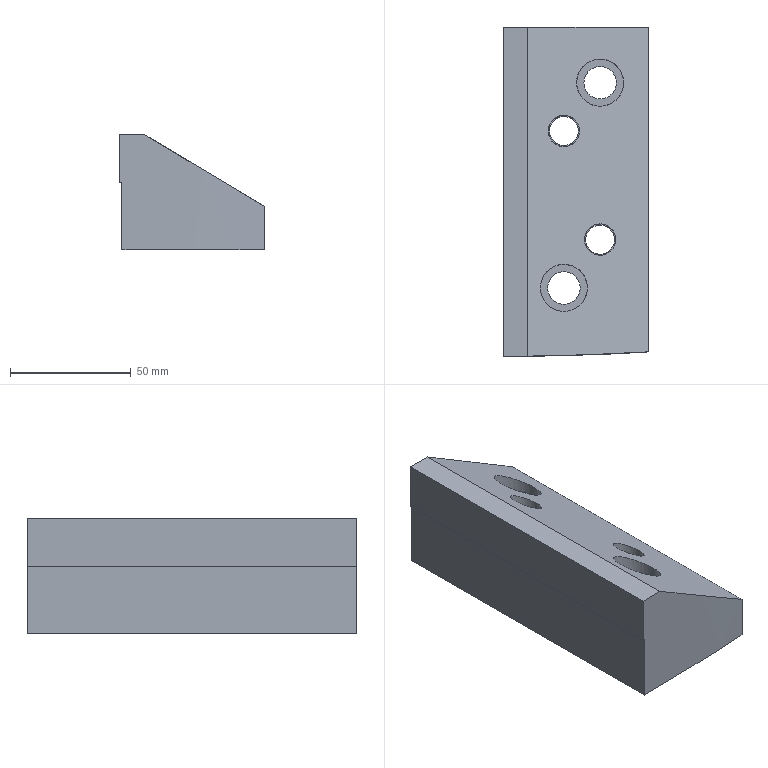Part | NX | features solid 2 | 1 solid | 21 faces | box 60 x 136.579 x 48 mm | volume 262854 mm3 | plane 12 | cylinder 8 | spline 1 | commonest cylinder face diameters 12 x2 13 x2 13.5 x2 19.5 x2
STEP:
#1=CARTESIAN_POINT('',(-70.,228.,-27.));
#2=VERTEX_POINT('',#1);
#3=CARTESIAN_POINT('',(-69.,228.,-27.));
#4=VERTEX_POINT('',#3);
#5=CARTESIAN_POINT('',(-470.374,228.,-27.));
#6=DIRECTION('',(-1.,0.,0.));
#7=VECTOR('',#6,1000.);
#8=LINE('',#5,#7);
#9=EDGE_CURVE('',#2,#4,#8,.F.);
#10=ORIENTED_EDGE('',*,*,#9,.F.);
#11=CARTESIAN_POINT('',(-70.,228.,-7.));
#12=VERTEX_POINT('',#11);
#13=CARTESIAN_POINT('',(-70.,228.,-67.));
#14=DIRECTION('',(0.,0.,1.));
#15=VECTOR('',#14,1000.);
#16=LINE('',#13,#15);
#17=EDGE_CURVE('',#2,#12,#16,.T.);
#18=ORIENTED_EDGE('',*,*,#17,.T.);
#19=CARTESIAN_POINT('',(-60.,228.,-7.));
#20=VERTEX_POINT('',#19);
#21=CARTESIAN_POINT('',(-470.374,228.,-7.));
#22=DIRECTION('',(1.,0.,0.));
#23=VECTOR('',#22,1000.);
#24=LINE('',#21,#23);
#25=EDGE_CURVE('',#12,#20,#24,.T.);
#26=ORIENTED_EDGE('',*,*,#25,.T.);
#27=CARTESIAN_POINT('',(-10.,228.,-37.));
#28=VERTEX_POINT('',#27);
#29=CARTESIAN_POINT('',(-60.,228.,-7.));
#30=DIRECTION('',(-0.8575,0.,0.5145));
#31=VECTOR('',#30,1000.);
#32=LINE('',#29,#31);
#33=EDGE_CURVE('',#28,#20,#32,.T.);
#34=ORIENTED_EDGE('',*,*,#33,.F.);
#35=CARTESIAN_POINT('',(-10.,228.,-55.));
#36=VERTEX_POINT('',#35);
#37=CARTESIAN_POINT('',(-10.,228.,-67.));
#38=DIRECTION('',(0.,0.,1.));
#39=VECTOR('',#38,1000.);
#40=LINE('',#37,#39);
#41=EDGE_CURVE('',#36,#28,#40,.T.);
#42=ORIENTED_EDGE('',*,*,#41,.F.);
#43=CARTESIAN_POINT('',(-69.,228.,-55.));
#44=VERTEX_POINT('',#43);
#45=CARTESIAN_POINT('',(-415.478,228.,-55.));
#46=DIRECTION('',(1.,0.,0.));
#47=VECTOR('',#46,1000.);
#48=LINE('',#45,#47);
#49=EDGE_CURVE('',#44,#36,#48,.T.);
#50=ORIENTED_EDGE('',*,*,#49,.F.);
#51=CARTESIAN_POINT('',(-69.,228.,-27.));
#52=DIRECTION('',(0.,0.,-1.));
#53=VECTOR('',#52,1000.);
#54=LINE('',#51,#53);
#55=EDGE_CURVE('',#4,#44,#54,.T.);
#56=ORIENTED_EDGE('',*,*,#55,.F.);
#57=EDGE_LOOP('',(#10,#18,#26,#34,#42,#50,#56));
#58=FACE_BOUND('',#57,.T.);
#59=CARTESIAN_POINT('',(-470.374,228.,-203.));
#60=DIRECTION('',(0.,-1.,0.));
#61=DIRECTION('',(1.,0.,0.));
#62=AXIS2_PLACEMENT_3D('',#59,#60,#61);
#63=PLANE('',#62);
#64=ADVANCED_FACE('',(#58),#63,.F.);
#65=CARTESIAN_POINT('',(-70.,91.421,-27.));
#66=VERTEX_POINT('',#65);
#67=CARTESIAN_POINT('',(-69.,91.45,-27.));
#68=VERTEX_POINT('',#67);
#69=CARTESIAN_POINT('',(-70.,91.421,-27.));
#70=CARTESIAN_POINT('',(-69.667,91.43,-27.));
#71=CARTESIAN_POINT('',(-69.333,91.44,-27.));
#72=CARTESIAN_POINT('',(-69.,91.45,-27.));
#73=B_SPLINE_CURVE_WITH_KNOTS('',3,(#69,#70,#71,#72),.UNSPECIFIED.,.F.,.F.,(4,4),(0.,0.001),.UNSPECIFIED.);
#74=EDGE_CURVE('',#66,#68,#73,.T.);
#75=ORIENTED_EDGE('',*,*,#74,.T.);
#76=CARTESIAN_POINT('',(-69.,91.45,-55.));
#77=VERTEX_POINT('',#76);
#78=CARTESIAN_POINT('',(-69.,91.45,-41.));
#79=DIRECTION('',(0.,0.,-1.));
#80=VECTOR('',#79,1000.);
#81=LINE('',#78,#80);
#82=EDGE_CURVE('',#68,#77,#81,.T.);
#83=ORIENTED_EDGE('',*,*,#82,.T.);
#84=CARTESIAN_POINT('',(-10.,93.522,-55.));
#85=VERTEX_POINT('',#84);
#86=CARTESIAN_POINT('',(-69.,91.45,-55.));
#87=CARTESIAN_POINT('',(-49.329,92.028,-55.));
#88=CARTESIAN_POINT('',(-29.641,92.101,-55.));
#89=CARTESIAN_POINT('',(-10.,93.522,-55.));
#90=B_SPLINE_CURVE_WITH_KNOTS('',3,(#86,#87,#88,#89),.UNSPECIFIED.,.F.,.F.,(4,4),(0.,0.05904),.UNSPECIFIED.);
#91=EDGE_CURVE('',#77,#85,#90,.T.);
#92=ORIENTED_EDGE('',*,*,#91,.T.);
#93=CARTESIAN_POINT('',(-10.,93.522,-37.));
#94=VERTEX_POINT('',#93);
#95=CARTESIAN_POINT('',(-10.,93.522,-46.));
#96=DIRECTION('',(0.,0.,-1.));
#97=VECTOR('',#96,1000.);
#98=LINE('',#95,#97);
#99=EDGE_CURVE('',#85,#94,#98,.F.);
#100=ORIENTED_EDGE('',*,*,#99,.T.);
#101=CARTESIAN_POINT('',(-60.,91.701,-7.));
#102=VERTEX_POINT('',#101);
#103=CARTESIAN_POINT('',(-60.,91.701,-7.));
#104=CARTESIAN_POINT('',(-43.328,92.124,-17.003));
#105=CARTESIAN_POINT('',(-26.651,92.317,-27.01));
#106=CARTESIAN_POINT('',(-10.,93.522,-37.));
#107=B_SPLINE_CURVE_WITH_KNOTS('',3,(#103,#104,#105,#106),.UNSPECIFIED.,.F.,.F.,(4,4),(0.,0.05834),.UNSPECIFIED.);
#108=EDGE_CURVE('',#102,#94,#107,.T.);
#109=ORIENTED_EDGE('',*,*,#108,.F.);
#110=CARTESIAN_POINT('',(-70.,91.421,-7.));
#111=VERTEX_POINT('',#110);
#112=CARTESIAN_POINT('',(-70.,91.421,-7.));
#113=CARTESIAN_POINT('',(-66.667,91.517,-7.));
#114=CARTESIAN_POINT('',(-63.334,91.617,-7.));
#115=CARTESIAN_POINT('',(-60.,91.701,-7.));
#116=B_SPLINE_CURVE_WITH_KNOTS('',3,(#112,#113,#114,#115),.UNSPECIFIED.,.F.,.F.,(4,4),(0.,0.01),.UNSPECIFIED.);
#117=EDGE_CURVE('',#111,#102,#116,.T.);
#118=ORIENTED_EDGE('',*,*,#117,.F.);
#119=CARTESIAN_POINT('',(-70.,91.421,-17.));
#120=DIRECTION('',(0.,0.,-1.));
#121=VECTOR('',#120,1000.);
#122=LINE('',#119,#121);
#123=EDGE_CURVE('',#66,#111,#122,.F.);
#124=ORIENTED_EDGE('',*,*,#123,.F.);
#125=EDGE_LOOP('',(#75,#83,#92,#100,#109,#118,#124));
#126=FACE_BOUND('',#125,.T.);
#127=CARTESIAN_POINT('',(-10.,93.522,-7.));
#128=CARTESIAN_POINT('',(-10.,93.522,-55.));
#129=CARTESIAN_POINT('',(-19.98,92.8,-7.));
#130=CARTESIAN_POINT('',(-19.98,92.8,-55.));
#131=CARTESIAN_POINT('',(-39.988,92.096,-7.));
#132=CARTESIAN_POINT('',(-39.988,92.096,-55.));
#133=CARTESIAN_POINT('',(-59.995,91.709,-7.));
#134=CARTESIAN_POINT('',(-59.995,91.709,-55.));
#135=CARTESIAN_POINT('',(-70.,91.421,-7.));
#136=CARTESIAN_POINT('',(-70.,91.421,-55.));
#137=B_SPLINE_SURFACE_WITH_KNOTS('',3,1,((#127,#128),(#129,#130),(#131,#132),(#133,#134),(#135,#136)),.SURF_OF_LINEAR_EXTRUSION.,.F.,.F.,.F.,(4,1,4),(2,2),(0.9515,0.9643,0.9772),(0.,1.),.UNSPECIFIED.);
#138=ADVANCED_FACE('',(#126),#137,.T.);
#139=ORIENTED_EDGE('',*,*,#123,.T.);
#140=CARTESIAN_POINT('',(-70.,99.381,-7.));
#141=DIRECTION('',(0.,1.,0.));
#142=VECTOR('',#141,1000.);
#143=LINE('',#140,#142);
#144=EDGE_CURVE('',#111,#12,#143,.T.);
#145=ORIENTED_EDGE('',*,*,#144,.T.);
#146=ORIENTED_EDGE('',*,*,#17,.F.);
#147=CARTESIAN_POINT('',(-70.,99.381,-27.));
#148=DIRECTION('',(0.,-1.,0.));
#149=VECTOR('',#148,1000.);
#150=LINE('',#147,#149);
#151=EDGE_CURVE('',#66,#2,#150,.F.);
#152=ORIENTED_EDGE('',*,*,#151,.F.);
#153=EDGE_LOOP('',(#139,#145,#146,#152));
#154=FACE_BOUND('',#153,.T.);
#155=CARTESIAN_POINT('',(-70.,99.381,-67.));
#156=DIRECTION('',(-1.,0.,0.));
#157=DIRECTION('',(0.,0.,1.));
#158=AXIS2_PLACEMENT_3D('',#155,#156,#157);
#159=PLANE('',#158);
#160=ADVANCED_FACE('',(#154),#159,.T.);
#161=CARTESIAN_POINT('',(-24.,140.,-55.));
#162=VERTEX_POINT('',#161);
#163=CARTESIAN_POINT('',(-30.,140.,-55.));
#164=DIRECTION('',(0.,0.,1.));
#165=DIRECTION('',(1.,0.,0.));
#166=AXIS2_PLACEMENT_3D('',#163,#164,#165);
#167=CIRCLE('',#166,6.);
#168=EDGE_CURVE('',#162,#162,#167,.T.);
#169=ORIENTED_EDGE('',*,*,#168,.T.);
#170=EDGE_LOOP('',(#169));
#171=FACE_BOUND('',#170,.T.);
#172=CARTESIAN_POINT('',(-39.,185.,-55.));
#173=VERTEX_POINT('',#172);
#174=CARTESIAN_POINT('',(-45.,185.,-55.));
#175=DIRECTION('',(0.,0.,1.));
#176=DIRECTION('',(1.,0.,0.));
#177=AXIS2_PLACEMENT_3D('',#174,#175,#176);
#178=CIRCLE('',#177,6.);
#179=EDGE_CURVE('',#173,#173,#178,.T.);
#180=ORIENTED_EDGE('',*,*,#179,.T.);
#181=EDGE_LOOP('',(#180));
#182=FACE_BOUND('',#181,.T.);
#183=CARTESIAN_POINT('',(-38.25,120.,-55.));
#184=VERTEX_POINT('',#183);
#185=CARTESIAN_POINT('',(-45.,120.,-55.));
#186=DIRECTION('',(0.,0.,1.));
#187=DIRECTION('',(1.,0.,0.));
#188=AXIS2_PLACEMENT_3D('',#185,#186,#187);
#189=CIRCLE('',#188,6.75);
#190=EDGE_CURVE('',#184,#184,#189,.T.);
#191=ORIENTED_EDGE('',*,*,#190,.T.);
#192=EDGE_LOOP('',(#191));
#193=FACE_BOUND('',#192,.T.);
#194=CARTESIAN_POINT('',(-23.25,205.,-55.));
#195=VERTEX_POINT('',#194);
#196=CARTESIAN_POINT('',(-30.,205.,-55.));
#197=DIRECTION('',(0.,0.,1.));
#198=DIRECTION('',(1.,0.,0.));
#199=AXIS2_PLACEMENT_3D('',#196,#197,#198);
#200=CIRCLE('',#199,6.75);
#201=EDGE_CURVE('',#195,#195,#200,.T.);
#202=ORIENTED_EDGE('',*,*,#201,.T.);
#203=EDGE_LOOP('',(#202));
#204=FACE_BOUND('',#203,.T.);
#205=ORIENTED_EDGE('',*,*,#49,.T.);
#206=CARTESIAN_POINT('',(-10.,99.381,-55.));
#207=DIRECTION('',(0.,1.,0.));
#208=VECTOR('',#207,1000.);
#209=LINE('',#206,#208);
#210=EDGE_CURVE('',#85,#36,#209,.T.);
#211=ORIENTED_EDGE('',*,*,#210,.F.);
#212=ORIENTED_EDGE('',*,*,#91,.F.);
#213=CARTESIAN_POINT('',(-69.,99.381,-55.));
#214=DIRECTION('',(0.,-1.,0.));
#215=VECTOR('',#214,1000.);
#216=LINE('',#213,#215);
#217=EDGE_CURVE('',#44,#77,#216,.T.);
#218=ORIENTED_EDGE('',*,*,#217,.F.);
#219=EDGE_LOOP('',(#205,#211,#212,#218));
#220=FACE_BOUND('',#219,.T.);
#221=CARTESIAN_POINT('',(-415.478,35.09,-55.));
#222=DIRECTION('',(0.,0.,1.));
#223=DIRECTION('',(1.,0.,0.));
#224=AXIS2_PLACEMENT_3D('',#221,#222,#223);
#225=PLANE('',#224);
#226=ADVANCED_FACE('',(#171,#182,#193,#204,#220),#225,.F.);
#227=ORIENTED_EDGE('',*,*,#25,.F.);
#228=ORIENTED_EDGE('',*,*,#144,.F.);
#229=ORIENTED_EDGE('',*,*,#117,.T.);
#230=CARTESIAN_POINT('',(-60.,99.381,-7.));
#231=DIRECTION('',(0.,-1.,0.));
#232=VECTOR('',#231,1000.);
#233=LINE('',#230,#232);
#234=EDGE_CURVE('',#20,#102,#233,.T.);
#235=ORIENTED_EDGE('',*,*,#234,.F.);
#236=EDGE_LOOP('',(#227,#228,#229,#235));
#237=FACE_BOUND('',#236,.T.);
#238=CARTESIAN_POINT('',(-70.,99.381,-7.));
#239=DIRECTION('',(0.,0.,-1.));
#240=DIRECTION('',(0.,1.,0.));
#241=AXIS2_PLACEMENT_3D('',#238,#239,#240);
#242=PLANE('',#241);
#243=ADVANCED_FACE('',(#237),#242,.F.);
#244=ORIENTED_EDGE('',*,*,#99,.F.);
#245=ORIENTED_EDGE('',*,*,#210,.T.);
#246=ORIENTED_EDGE('',*,*,#41,.T.);
#247=CARTESIAN_POINT('',(-10.,99.381,-37.));
#248=DIRECTION('',(0.,1.,0.));
#249=VECTOR('',#248,1000.);
#250=LINE('',#247,#249);
#251=EDGE_CURVE('',#94,#28,#250,.T.);
#252=ORIENTED_EDGE('',*,*,#251,.F.);
#253=EDGE_LOOP('',(#244,#245,#246,#252));
#254=FACE_BOUND('',#253,.T.);
#255=CARTESIAN_POINT('',(-10.,99.381,-67.));
#256=DIRECTION('',(-1.,0.,0.));
#257=DIRECTION('',(0.,0.,1.));
#258=AXIS2_PLACEMENT_3D('',#255,#256,#257);
#259=PLANE('',#258);
#260=ADVANCED_FACE('',(#254),#259,.F.);
#261=CARTESIAN_POINT('',(-36.5,140.,-21.1));
#262=VERTEX_POINT('',#261);
#263=CARTESIAN_POINT('',(-30.,140.,-25.));
#264=DIRECTION('',(-0.5145,0.,-0.8575));
#265=DIRECTION('',(-0.8575,0.,0.5145));
#266=AXIS2_PLACEMENT_3D('',#263,#264,#265);
#267=ELLIPSE('',#266,7.58,6.5);
#268=EDGE_CURVE('',#262,#262,#267,.T.);
#269=ORIENTED_EDGE('',*,*,#268,.T.);
#270=EDGE_LOOP('',(#269));
#271=FACE_BOUND('',#270,.T.);
#272=CARTESIAN_POINT('',(-51.5,185.,-12.1));
#273=VERTEX_POINT('',#272);
#274=CARTESIAN_POINT('',(-45.,185.,-16.));
#275=DIRECTION('',(-0.5145,0.,-0.8575));
#276=DIRECTION('',(-0.8575,0.,0.5145));
#277=AXIS2_PLACEMENT_3D('',#274,#275,#276);
#278=ELLIPSE('',#277,7.58,6.5);
#279=EDGE_CURVE('',#273,#273,#278,.T.);
#280=ORIENTED_EDGE('',*,*,#279,.T.);
#281=EDGE_LOOP('',(#280));
#282=FACE_BOUND('',#281,.T.);
#283=CARTESIAN_POINT('',(-54.75,120.,-10.15));
#284=VERTEX_POINT('',#283);
#285=CARTESIAN_POINT('',(-45.,120.,-16.));
#286=DIRECTION('',(-0.5145,0.,-0.8575));
#287=DIRECTION('',(-0.8575,0.,0.5145));
#288=AXIS2_PLACEMENT_3D('',#285,#286,#287);
#289=ELLIPSE('',#288,11.37,9.75);
#290=EDGE_CURVE('',#284,#284,#289,.T.);
#291=ORIENTED_EDGE('',*,*,#290,.T.);
#292=EDGE_LOOP('',(#291));
#293=FACE_BOUND('',#292,.T.);
#294=CARTESIAN_POINT('',(-39.75,205.,-19.15));
#295=VERTEX_POINT('',#294);
#296=CARTESIAN_POINT('',(-30.,205.,-25.));
#297=DIRECTION('',(-0.5145,0.,-0.8575));
#298=DIRECTION('',(-0.8575,0.,0.5145));
#299=AXIS2_PLACEMENT_3D('',#296,#297,#298);
#300=ELLIPSE('',#299,11.37,9.75);
#301=EDGE_CURVE('',#295,#295,#300,.T.);
#302=ORIENTED_EDGE('',*,*,#301,.T.);
#303=EDGE_LOOP('',(#302));
#304=FACE_BOUND('',#303,.T.);
#305=ORIENTED_EDGE('',*,*,#33,.T.);
#306=ORIENTED_EDGE('',*,*,#234,.T.);
#307=ORIENTED_EDGE('',*,*,#108,.T.);
#308=ORIENTED_EDGE('',*,*,#251,.T.);
#309=EDGE_LOOP('',(#305,#306,#307,#308));
#310=FACE_BOUND('',#309,.T.);
#311=CARTESIAN_POINT('',(-60.,232.,-7.));
#312=DIRECTION('',(-0.5145,0.,-0.8575));
#313=DIRECTION('',(-0.8575,0.,0.5145));
#314=AXIS2_PLACEMENT_3D('',#311,#312,#313);
#315=PLANE('',#314);
#316=ADVANCED_FACE('',(#271,#282,#293,#304,#310),#315,.F.);
#317=ORIENTED_EDGE('',*,*,#55,.T.);
#318=ORIENTED_EDGE('',*,*,#217,.T.);
#319=ORIENTED_EDGE('',*,*,#82,.F.);
#320=CARTESIAN_POINT('',(-69.,99.381,-27.));
#321=DIRECTION('',(0.,-1.,0.));
#322=VECTOR('',#321,1000.);
#323=LINE('',#320,#322);
#324=EDGE_CURVE('',#68,#4,#323,.F.);
#325=ORIENTED_EDGE('',*,*,#324,.T.);
#326=EDGE_LOOP('',(#317,#318,#319,#325));
#327=FACE_BOUND('',#326,.T.);
#328=CARTESIAN_POINT('',(-69.,99.381,-27.));
#329=DIRECTION('',(1.,0.,0.));
#330=DIRECTION('',(0.,0.,-1.));
#331=AXIS2_PLACEMENT_3D('',#328,#329,#330);
#332=PLANE('',#331);
#333=ADVANCED_FACE('',(#327),#332,.F.);
#334=ORIENTED_EDGE('',*,*,#74,.F.);
#335=ORIENTED_EDGE('',*,*,#151,.T.);
#336=ORIENTED_EDGE('',*,*,#9,.T.);
#337=ORIENTED_EDGE('',*,*,#324,.F.);
#338=EDGE_LOOP('',(#334,#335,#336,#337));
#339=FACE_BOUND('',#338,.T.);
#340=CARTESIAN_POINT('',(-70.,99.381,-27.));
#341=DIRECTION('',(0.,0.,1.));
#342=DIRECTION('',(0.,1.,0.));
#343=AXIS2_PLACEMENT_3D('',#340,#341,#342);
#344=PLANE('',#343);
#345=ADVANCED_FACE('',(#339),#344,.F.);
#346=CARTESIAN_POINT('',(-36.75,205.,-35.));
#347=VERTEX_POINT('',#346);
#348=CARTESIAN_POINT('',(-30.,205.,-35.));
#349=DIRECTION('',(0.,0.,-1.));
#350=DIRECTION('',(-1.,0.,0.));
#351=AXIS2_PLACEMENT_3D('',#348,#349,#350);
#352=CIRCLE('',#351,6.75);
#353=EDGE_CURVE('',#347,#347,#352,.F.);
#354=ORIENTED_EDGE('',*,*,#353,.T.);
#355=EDGE_LOOP('',(#354));
#356=FACE_BOUND('',#355,.T.);
#357=ORIENTED_EDGE('',*,*,#201,.F.);
#358=EDGE_LOOP('',(#357));
#359=FACE_BOUND('',#358,.T.);
#360=CARTESIAN_POINT('',(-30.,205.,-75.));
#361=DIRECTION('',(0.,0.,1.));
#362=DIRECTION('',(1.,0.,0.));
#363=AXIS2_PLACEMENT_3D('',#360,#361,#362);
#364=CYLINDRICAL_SURFACE('',#363,6.75);
#365=ADVANCED_FACE('',(#356,#359),#364,.F.);
#366=CARTESIAN_POINT('',(-20.25,205.,-35.));
#367=VERTEX_POINT('',#366);
#368=CARTESIAN_POINT('',(-30.,205.,-35.));
#369=DIRECTION('',(0.,0.,1.));
#370=DIRECTION('',(1.,0.,0.));
#371=AXIS2_PLACEMENT_3D('',#368,#369,#370);
#372=CIRCLE('',#371,9.75);
#373=EDGE_CURVE('',#367,#367,#372,.T.);
#374=ORIENTED_EDGE('',*,*,#373,.F.);
#375=EDGE_LOOP('',(#374));
#376=FACE_BOUND('',#375,.T.);
#377=ORIENTED_EDGE('',*,*,#301,.F.);
#378=EDGE_LOOP('',(#377));
#379=FACE_BOUND('',#378,.T.);
#380=CARTESIAN_POINT('',(-30.,205.,-35.));
#381=DIRECTION('',(0.,0.,1.));
#382=DIRECTION('',(1.,0.,0.));
#383=AXIS2_PLACEMENT_3D('',#380,#381,#382);
#384=CYLINDRICAL_SURFACE('',#383,9.75);
#385=ADVANCED_FACE('',(#376,#379),#384,.F.);
#386=ORIENTED_EDGE('',*,*,#353,.F.);
#387=EDGE_LOOP('',(#386));
#388=FACE_BOUND('',#387,.T.);
#389=ORIENTED_EDGE('',*,*,#373,.T.);
#390=EDGE_LOOP('',(#389));
#391=FACE_BOUND('',#390,.T.);
#392=CARTESIAN_POINT('',(-30.,200.,-35.));
#393=DIRECTION('',(0.,0.,-1.));
#394=DIRECTION('',(-1.,0.,0.));
#395=AXIS2_PLACEMENT_3D('',#392,#393,#394);
#396=PLANE('',#395);
#397=ADVANCED_FACE('',(#388,#391),#396,.F.);
#398=CARTESIAN_POINT('',(-51.75,120.,-35.));
#399=VERTEX_POINT('',#398);
#400=CARTESIAN_POINT('',(-45.,120.,-35.));
#401=DIRECTION('',(0.,0.,-1.));
#402=DIRECTION('',(-1.,0.,0.));
#403=AXIS2_PLACEMENT_3D('',#400,#401,#402);
#404=CIRCLE('',#403,6.75);
#405=EDGE_CURVE('',#399,#399,#404,.F.);
#406=ORIENTED_EDGE('',*,*,#405,.T.);
#407=EDGE_LOOP('',(#406));
#408=FACE_BOUND('',#407,.T.);
#409=ORIENTED_EDGE('',*,*,#190,.F.);
#410=EDGE_LOOP('',(#409));
#411=FACE_BOUND('',#410,.T.);
#412=CARTESIAN_POINT('',(-45.,120.,-75.));
#413=DIRECTION('',(0.,0.,1.));
#414=DIRECTION('',(1.,0.,0.));
#415=AXIS2_PLACEMENT_3D('',#412,#413,#414);
#416=CYLINDRICAL_SURFACE('',#415,6.75);
#417=ADVANCED_FACE('',(#408,#411),#416,.F.);
#418=CARTESIAN_POINT('',(-35.25,120.,-35.));
#419=VERTEX_POINT('',#418);
#420=CARTESIAN_POINT('',(-45.,120.,-35.));
#421=DIRECTION('',(0.,0.,1.));
#422=DIRECTION('',(1.,0.,0.));
#423=AXIS2_PLACEMENT_3D('',#420,#421,#422);
#424=CIRCLE('',#423,9.75);
#425=EDGE_CURVE('',#419,#419,#424,.T.);
#426=ORIENTED_EDGE('',*,*,#425,.F.);
#427=EDGE_LOOP('',(#426));
#428=FACE_BOUND('',#427,.T.);
#429=ORIENTED_EDGE('',*,*,#290,.F.);
#430=EDGE_LOOP('',(#429));
#431=FACE_BOUND('',#430,.T.);
#432=CARTESIAN_POINT('',(-45.,120.,-35.));
#433=DIRECTION('',(0.,0.,1.));
#434=DIRECTION('',(1.,0.,0.));
#435=AXIS2_PLACEMENT_3D('',#432,#433,#434);
#436=CYLINDRICAL_SURFACE('',#435,9.75);
#437=ADVANCED_FACE('',(#428,#431),#436,.F.);
#438=ORIENTED_EDGE('',*,*,#405,.F.);
#439=EDGE_LOOP('',(#438));
#440=FACE_BOUND('',#439,.T.);
#441=ORIENTED_EDGE('',*,*,#425,.T.);
#442=EDGE_LOOP('',(#441));
#443=FACE_BOUND('',#442,.T.);
#444=CARTESIAN_POINT('',(-45.,120.,-35.));
#445=DIRECTION('',(0.,0.,-1.));
#446=DIRECTION('',(-1.,0.,0.));
#447=AXIS2_PLACEMENT_3D('',#444,#445,#446);
#448=PLANE('',#447);
#449=ADVANCED_FACE('',(#440,#443),#448,.F.);
#450=CARTESIAN_POINT('',(-51.,185.,-35.));
#451=VERTEX_POINT('',#450);
#452=CARTESIAN_POINT('',(-45.,185.,-35.));
#453=DIRECTION('',(0.,0.,-1.));
#454=DIRECTION('',(-1.,0.,0.));
#455=AXIS2_PLACEMENT_3D('',#452,#453,#454);
#456=CIRCLE('',#455,6.);
#457=EDGE_CURVE('',#451,#451,#456,.F.);
#458=ORIENTED_EDGE('',*,*,#457,.T.);
#459=EDGE_LOOP('',(#458));
#460=FACE_BOUND('',#459,.T.);
#461=ORIENTED_EDGE('',*,*,#179,.F.);
#462=EDGE_LOOP('',(#461));
#463=FACE_BOUND('',#462,.T.);
#464=CARTESIAN_POINT('',(-45.,185.,-75.));
#465=DIRECTION('',(0.,0.,1.));
#466=DIRECTION('',(1.,0.,0.));
#467=AXIS2_PLACEMENT_3D('',#464,#465,#466);
#468=CYLINDRICAL_SURFACE('',#467,6.);
#469=ADVANCED_FACE('',(#460,#463),#468,.F.);
#470=CARTESIAN_POINT('',(-38.5,185.,-35.));
#471=VERTEX_POINT('',#470);
#472=CARTESIAN_POINT('',(-45.,185.,-35.));
#473=DIRECTION('',(0.,0.,1.));
#474=DIRECTION('',(1.,0.,0.));
#475=AXIS2_PLACEMENT_3D('',#472,#473,#474);
#476=CIRCLE('',#475,6.5);
#477=EDGE_CURVE('',#471,#471,#476,.T.);
#478=ORIENTED_EDGE('',*,*,#477,.F.);
#479=EDGE_LOOP('',(#478));
#480=FACE_BOUND('',#479,.T.);
#481=ORIENTED_EDGE('',*,*,#279,.F.);
#482=EDGE_LOOP('',(#481));
#483=FACE_BOUND('',#482,.T.);
#484=CARTESIAN_POINT('',(-45.,185.,-35.));
#485=DIRECTION('',(0.,0.,1.));
#486=DIRECTION('',(1.,0.,0.));
#487=AXIS2_PLACEMENT_3D('',#484,#485,#486);
#488=CYLINDRICAL_SURFACE('',#487,6.5);
#489=ADVANCED_FACE('',(#480,#483),#488,.F.);
#490=ORIENTED_EDGE('',*,*,#457,.F.);
#491=EDGE_LOOP('',(#490));
#492=FACE_BOUND('',#491,.T.);
#493=ORIENTED_EDGE('',*,*,#477,.T.);
#494=EDGE_LOOP('',(#493));
#495=FACE_BOUND('',#494,.T.);
#496=CARTESIAN_POINT('',(-45.,180.,-35.));
#497=DIRECTION('',(0.,0.,-1.));
#498=DIRECTION('',(-1.,0.,0.));
#499=AXIS2_PLACEMENT_3D('',#496,#497,#498);
#500=PLANE('',#499);
#501=ADVANCED_FACE('',(#492,#495),#500,.F.);
#502=CARTESIAN_POINT('',(-36.,140.,-35.));
#503=VERTEX_POINT('',#502);
#504=CARTESIAN_POINT('',(-30.,140.,-35.));
#505=DIRECTION('',(0.,0.,-1.));
#506=DIRECTION('',(-1.,0.,0.));
#507=AXIS2_PLACEMENT_3D('',#504,#505,#506);
#508=CIRCLE('',#507,6.);
#509=EDGE_CURVE('',#503,#503,#508,.F.);
#510=ORIENTED_EDGE('',*,*,#509,.T.);
#511=EDGE_LOOP('',(#510));
#512=FACE_BOUND('',#511,.T.);
#513=ORIENTED_EDGE('',*,*,#168,.F.);
#514=EDGE_LOOP('',(#513));
#515=FACE_BOUND('',#514,.T.);
#516=CARTESIAN_POINT('',(-30.,140.,-75.));
#517=DIRECTION('',(0.,0.,1.));
#518=DIRECTION('',(1.,0.,0.));
#519=AXIS2_PLACEMENT_3D('',#516,#517,#518);
#520=CYLINDRICAL_SURFACE('',#519,6.);
#521=ADVANCED_FACE('',(#512,#515),#520,.F.);
#522=CARTESIAN_POINT('',(-23.5,140.,-35.));
#523=VERTEX_POINT('',#522);
#524=CARTESIAN_POINT('',(-30.,140.,-35.));
#525=DIRECTION('',(0.,0.,1.));
#526=DIRECTION('',(1.,0.,0.));
#527=AXIS2_PLACEMENT_3D('',#524,#525,#526);
#528=CIRCLE('',#527,6.5);
#529=EDGE_CURVE('',#523,#523,#528,.T.);
#530=ORIENTED_EDGE('',*,*,#529,.F.);
#531=EDGE_LOOP('',(#530));
#532=FACE_BOUND('',#531,.T.);
#533=ORIENTED_EDGE('',*,*,#268,.F.);
#534=EDGE_LOOP('',(#533));
#535=FACE_BOUND('',#534,.T.);
#536=CARTESIAN_POINT('',(-30.,140.,-35.));
#537=DIRECTION('',(0.,0.,1.));
#538=DIRECTION('',(1.,0.,0.));
#539=AXIS2_PLACEMENT_3D('',#536,#537,#538);
#540=CYLINDRICAL_SURFACE('',#539,6.5);
#541=ADVANCED_FACE('',(#532,#535),#540,.F.);
#542=ORIENTED_EDGE('',*,*,#509,.F.);
#543=EDGE_LOOP('',(#542));
#544=FACE_BOUND('',#543,.T.);
#545=ORIENTED_EDGE('',*,*,#529,.T.);
#546=EDGE_LOOP('',(#545));
#547=FACE_BOUND('',#546,.T.);
#548=CARTESIAN_POINT('',(-30.,140.,-35.));
#549=DIRECTION('',(0.,0.,-1.));
#550=DIRECTION('',(-1.,0.,0.));
#551=AXIS2_PLACEMENT_3D('',#548,#549,#550);
#552=PLANE('',#551);
#553=ADVANCED_FACE('',(#544,#547),#552,.F.);
#554=CLOSED_SHELL('',(#64,#138,#160,#226,#243,#260,#316,#333,#345,#365,#385,#397,#417,#437,#449,#469,#489,#501,#521,#541,#553));
#555=MANIFOLD_SOLID_BREP('',#554);
#556=(LENGTH_UNIT()NAMED_UNIT(*)SI_UNIT(.MILLI.,.METRE.));
#557=UNCERTAINTY_MEASURE_WITH_UNIT(LENGTH_MEASURE(0.0508),#556,'','');
#558=(NAMED_UNIT(*)PLANE_ANGLE_UNIT()SI_UNIT($,.RADIAN.));
#559=(NAMED_UNIT(*)SI_UNIT($,.STERADIAN.)SOLID_ANGLE_UNIT());
#560=(GEOMETRIC_REPRESENTATION_CONTEXT(3)GLOBAL_UNCERTAINTY_ASSIGNED_CONTEXT((#557))GLOBAL_UNIT_ASSIGNED_CONTEXT((#556,#558,#559))REPRESENTATION_CONTEXT('',''));
#561=ADVANCED_BREP_SHAPE_REPRESENTATION('',(#555),#560);